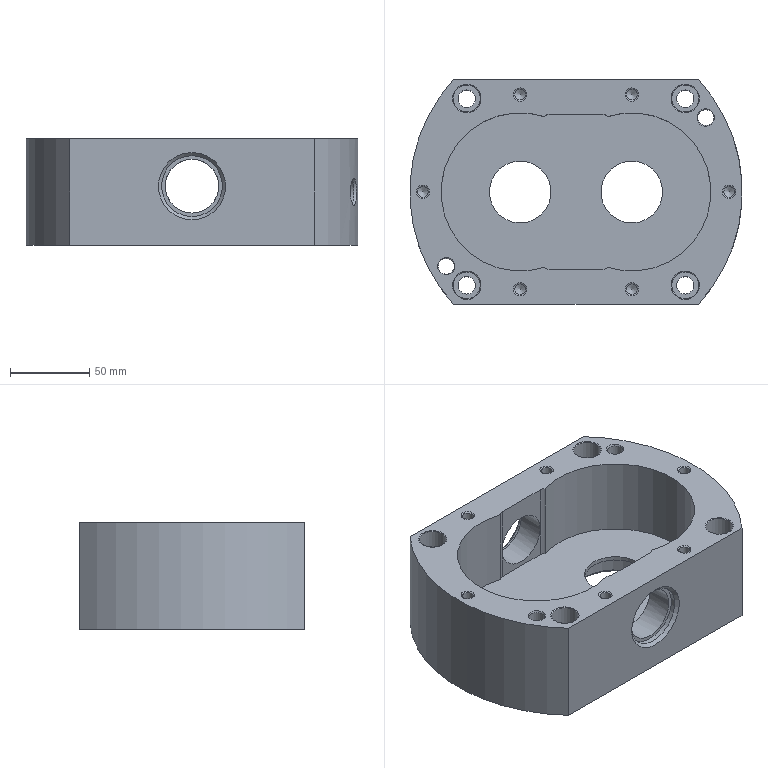NC program | NX | posted with a generic post | part box 210 x 142 x 67.4 mm
Whole program:
N10 G17 G21 G94 G90
(FLOOR_WALL , TOOL : D50)
N12 T02 M6
N14 G54
N16 G17 G0 G90 X-46.563 Y43.697 B0. C0. S1200 M3
N18 G43 Z30. H2
N20 Z2.65
N22 G94 G1 Z-0.35 F1000.
N24 X-43.563
N26 X43.563 F2000.
N28 Y9.999
N30 X-43.563
N32 Y-23.7
N34 X43.563
N36 X46.563
N38 Z2.65
N40 G0 Z30.
N42 X-50.098 Y43.697
N44 Z2.301
N46 G1 Z-0.699 F1000.
N48 X-47.098
N50 X47.098 F2000.
N52 Y9.999
N54 X-47.098
N56 Y-23.7
N58 X47.098
N60 X50.098
N62 Z2.301
N64 G0 Z30.
N66 X-52.803 Y43.697
N68 Z1.951
N70 G1 Z-1.049 F1000.
N72 X-49.803
N74 X49.803 F2000.
N76 Y9.999
N78 X-49.803
N80 Y-23.7
N82 X49.803
N84 X52.803
N86 Z1.951
N88 G0 Z30.
N90 X-55.078 Y43.697
N92 Z1.602
N94 G1 Z-1.398 F1000.
N96 X-52.078
N98 X52.078 F2000.
N100 Y9.999
N102 X-52.078
N104 Y-23.7
N106 X52.078
N108 X55.078
N110 Z1.602
N112 G0 Z30.
N114 X-57.078 Y43.697
N116 Z1.252
N118 G1 Z-1.748 F1000.
N120 X-54.078
N122 X54.078 F2000.
N124 Y9.999
N126 X-54.078
N128 Y-23.7
N130 X54.078
N132 X57.078
N134 Z1.252
N136 G0 Z30.
N138 X-58.881 Y43.697
N140 Z0.903
N142 G1 Z-2.097 F1000.
N144 X-55.881
N146 X55.881 F2000.
N148 Y9.999
N150 X-55.881
N152 Y-23.7
N154 X55.881
N156 X58.881
N158 Z0.903
N160 G0 Z30.
N162 X-60.535 Y43.697
N164 Z0.553
N166 G1 Z-2.447 F1000.
N168 X-57.535
N170 X57.535 F2000.
N172 Y9.999
N174 X-57.535
N176 Y-23.7
N178 X57.535
N180 X60.535
N182 Z0.553
N184 G0 Z30.
N186 X-62.07 Y43.697
N188 Z0.204
N190 G1 Z-2.796 F1000.
N192 X-59.07
N194 X59.07 F2000.
N196 Y9.999
N198 X-59.07
N200 Y-23.7
N202 X59.07
N204 X62.07
N206 Z0.204
N208 G0 Z30.
N210 X-63.509 Y43.697
N212 Z-0.146
N214 G1 Z-3.146 F1000.
N216 X-60.509
N218 X60.509 F2000.
N220 Y9.999
N222 X-60.509
N224 Y-23.7
N226 X60.509
N228 X63.509
N230 Z-0.146
N232 G0 Z30.
N234 X-64.866 Y43.697
N236 Z-0.495
N238 G1 Z-3.495 F1000.
N240 X-61.866
N242 X61.866 F2000.
N244 Y9.999
N246 X-61.866
N248 Y-23.7
N250 X61.866
N252 X64.866
N254 Z-0.495
N256 G0 Z30.
N258 X-66.153 Y43.697
N260 Z-0.845
N262 G1 Z-3.845 F1000.
N264 X-63.153
N266 X63.153 F2000.
N268 Y9.999
N270 X-63.153
N272 Y-23.7
N274 X63.153
N276 X66.153
N278 Z-0.845
N280 G0 Z30.
N282 X-67.38 Y43.697
N284 Z-1.194
N286 G1 Z-4.194 F1000.
N288 X-64.38
N290 X64.38 F2000.
N292 Y9.999
N294 X-64.38
N296 Y-23.7
N298 X64.38
N300 X67.38
N302 Z-1.194
N304 G0 Z30.
N306 X-68.553 Y43.697
N308 Z-1.544
N310 G1 Z-4.544 F1000.
N312 X-65.553
N314 X65.553 F2000.
N316 Y9.999
N318 X-65.553
N320 Y-23.7
N322 X65.553
N324 X68.553
N326 Z-1.544
N328 G0 Z30.
N330 X-69.68 Y43.697
N332 Z-1.893
N334 G1 Z-4.893 F1000.
N336 X-66.68
N338 X66.68 F2000.
N340 Y9.999
N342 X-66.68
N344 Y-23.7
N346 X66.68
N348 X69.68
N350 Z-1.893
N352 G0 Z30.
N354 X-70.763 Y43.697
N356 Z-2.243
N358 G1 Z-5.243 F1000.
N360 X-67.763
N362 X67.763 F2000.
N364 Y9.999
N366 X-67.763
N368 Y-23.7
N370 X67.763
N372 X70.763
N374 Z-2.243
N376 G0 Z30.
N378 X-71.809 Y43.697
N380 Z-2.592
N382 G1 Z-5.592 F1000.
N384 X-68.809
N386 X68.809 F2000.
N388 Y9.999
N390 X-68.809
N392 Y-23.7
N394 X68.809
N396 X71.809
N398 Z-2.592
N400 G0 Z30.
N402 X-72.82 Y43.697
N404 Z-2.941
N406 G1 Z-5.941 F1000.
N408 X-69.82
N410 X69.82 F2000.
N412 Y9.999
N414 X-69.82
N416 Y-23.7
N418 X69.82
N420 X72.82
N422 Z-2.941
N424 G0 Z30.
N426 X-73.798 Y43.697
N428 Z-3.291
N430 G1 Z-6.291 F1000.
N432 X-70.798
N434 X70.798 F2000.
N436 Y9.999
N438 X-70.798
N440 Y-23.7
N442 X70.798
N444 X73.798
N446 Z-3.291
N448 G0 Z30.
N450 X-74.748 Y43.697
N452 Z-3.64
N454 G1 Z-6.64 F1000.
N456 X-71.748
N458 X71.748 F2000.
N460 Y9.999
N462 X-71.748
N464 Y-23.7
N466 X71.748
N468 X74.748
N470 Z-3.64
N472 G0 Z30.
N474 X-75.67 Y43.697
N476 Z-3.99
N478 G1 Z-6.99 F1000.
N480 X-72.67
N482 X72.67 F2000.
N484 Y9.999
N486 X-72.67
N488 Y-23.7
N490 X72.67
N492 X75.67
N494 Z-3.99
N496 G0 Z30.
N498 X-76.567 Y43.697
N500 Z-4.339
N502 G1 Z-7.339 F1000.
N504 X-73.567
N506 X73.567 F2000.
N508 Y9.999
N510 X-73.567
N512 Y-23.7
N514 X73.567
N516 X76.567
N518 Z-4.339
N520 G0 Z30.
N522 X-77.44 Y43.697
N524 Z-4.689
N526 G1 Z-7.689 F1000.
N528 X-74.44
N530 X74.44 F2000.
N532 Y9.999
N534 X-74.44
N536 Y-23.7
N538 X74.44
N540 X77.44
N542 Z-4.689
N544 G0 Z30.
N546 X-78.292 Y43.697
N548 Z-5.038
N550 G1 Z-8.038 F1000.
N552 X-75.292
N554 X75.292 F2000.
N556 Y9.999
N558 X-75.292
N560 Y-23.7
N562 X75.292
N564 X78.292
N566 Z-5.038
N568 G0 Z30.
N570 X-79.123 Y43.697
N572 Z-5.388
N574 G1 Z-8.388 F1000.
N576 X-76.123
N578 X76.123 F2000.
N580 Y9.999
N582 X-76.123
N584 Y-23.7
N586 X76.123
N588 X79.123
N590 Z-5.388
N592 G0 Z30.
N594 X-79.934 Y43.697
N596 Z-5.737
N598 G1 Z-8.737 F1000.
N600 X-76.934
N602 X76.934 F2000.
N604 Y9.999
N606 X-76.934
N608 Y-23.7
N610 X76.934
N612 X79.934
N614 Z-5.737
N616 G0 Z30.
N618 X-80.728 Y43.697
N620 Z-6.087
N622 G1 Z-9.087 F1000.
N624 X-77.728
N626 X77.728 F2000.
N628 Y9.999
N630 X-77.728
N632 Y-23.7
N634 X77.728
N636 X80.728
N638 Z-6.087
N640 G0 Z30.
N642 X-81.504 Y43.697
N644 Z-6.436
N646 G1 Z-9.436 F1000.
N648 X-78.504
N650 X78.504 F2000.
N652 Y9.999
N654 X-78.504
N656 Y-23.7
N658 X78.504
N660 X81.504
N662 Z-6.436
N664 G0 Z30.
N666 X-82.263 Y43.697
N668 Z-6.786
N670 G1 Z-9.786 F1000.
N672 X-79.263
N674 X79.263 F2000.
N676 Y9.999
N678 X-79.263
N680 Y-23.7
N682 X79.263
N684 X82.263
N686 Z-6.786
N688 G0 Z30.
N690 X-83.008 Y43.697
N692 Z-7.135
N694 G1 Z-10.135 F1000.
N696 X-80.008
N698 X80.008 F2000.
N700 Y9.999
N702 X-80.008
N704 Y-23.7
N706 X80.008
N708 X83.008
N710 Z-7.135
N712 G0 Z30.
N714 X-83.737 Y43.697
N716 Z-7.485
N718 G1 Z-10.485 F1000.
N720 X-80.737
N722 X80.737 F2000.
N724 Y9.999
N726 X-80.737
N728 Y-23.7
N730 X80.737
N732 X83.737
N734 Z-7.485
N736 G0 Z30.
N738 X-84.452 Y43.697
N740 Z-7.834
N742 G1 Z-10.834 F1000.
N744 X-81.452
N746 X81.452 F2000.
N748 Y9.999
N750 X-81.452
N752 Y-23.7
N754 X81.452
N756 X84.452
N758 Z-7.834
N760 G0 Z30.
N762 X-85.154 Y43.697
N764 Z-8.184
N766 G1 Z-11.184 F1000.
N768 X-82.154
N770 X82.154 F2000.
N772 Y9.999
N774 X-82.154
N776 Y-23.7
N778 X82.154
N780 X85.154
N782 Z-8.184
N784 G0 Z30.
N786 X-85.843 Y43.697
N788 Z-8.533
N790 G1 Z-11.533 F1000.
N792 X-82.843
N794 X82.843 F2000.
N796 Y9.999
N798 X-82.843
N800 Y-23.7
N802 X82.843
N804 X85.843
N806 Z-8.533
N808 G0 Z30.
N810 X-86.52 Y43.697
N812 Z-8.883
N814 G1 Z-11.883 F1000.
N816 X-83.52
N818 X83.52 F2000.
N820 Y9.999
N822 X-83.52
N824 Y-23.7
N826 X83.52
N828 X86.52
N830 Z-8.883
N832 G0 Z30.
N834 X-87.185 Y43.697
N836 Z-9.232
N838 G1 Z-12.232 F1000.
N840 X-84.185
N842 X84.185 F2000.
N844 Y9.999
N846 X-84.185
N848 Y-23.7
N850 X84.185
N852 X87.185
N854 Z-9.232
N856 G0 Z30.
N858 X-87.838 Y43.697
N860 Z-9.582
N862 G1 Z-12.582 F1000.
N864 X-84.838
N866 X84.838 F2000.
N868 Y9.999
N870 X-84.838
N872 Y-23.7
N874 X84.838
N876 X87.838
N878 Z-9.582
N880 G0 Z30.
N882 X-88.481 Y43.697
N884 Z-9.931
N886 G1 Z-12.931 F1000.
N888 X-85.481
N890 X85.481 F2000.
N892 Y9.999
N894 X-85.481
N896 Y-23.7
N898 X85.481
N900 X88.481
N902 Z-9.931
N904 G0 Z30.
N906 X-89.113 Y43.697
N908 Z-10.281
N910 G1 Z-13.281 F1000.
N912 X-86.113
N914 X86.113 F2000.
N916 Y9.999
N918 X-86.113
N920 Y-23.7
N922 X86.113
N924 X89.113
N926 Z-10.281
N928 G0 Z30.
N930 X-89.735 Y43.697
N932 Z-10.63
N934 G1 Z-13.63 F1000.
N936 X-86.735
N938 X86.735 F2000.
N940 Y9.999
N942 X-86.735
N944 Y-23.7
N946 X86.735
N948 X89.735
N950 Z-10.63
N952 G0 Z30.
N954 X-90.348 Y43.697
N956 Z-10.98
N958 G1 Z-13.98 F1000.
N960 X-87.348
N962 X87.348 F2000.
N964 Y9.999
N966 X-87.348
N968 Y-23.7
N970 X87.348
N972 X90.348
N974 Z-10.98
N976 G0 Z30.
N978 X-90.951 Y43.697
N980 Z-11.329
N982 G1 Z-14.329 F1000.
N984 X-87.951
N986 X87.951 F2000.
N988 Y9.999
N990 X-87.951
N992 Y-23.7
N994 X87.951
N996 X90.951
N998 Z-11.329
N1000 G0 Z30.
N1002 X-91.545 Y43.697
N1004 Z-11.679
N1006 G1 Z-14.679 F1000.
N1008 X-88.545
N1010 X88.545 F2000.
N1012 Y9.999
N1014 X-88.545
N1016 Y-23.7
N1018 X88.545
N1020 X91.545
N1022 Z-11.679
N1024 G0 Z30.
N1026 X-92.13 Y43.697
N1028 Z-12.028
N1030 G1 Z-15.028 F1000.
N1032 X-89.13
N1034 X89.13 F2000.
N1036 Y9.999
N1038 X-89.13
N1040 Y-23.7
N1042 X89.13
N1044 X92.13
N1046 Z-12.028
N1048 G0 Z30.
N1050 X-92.707 Y43.697
N1052 Z-12.377
N1054 G1 Z-15.377 F1000.
N1056 X-89.707
N1058 X89.707 F2000.
N1060 Y9.999
N1062 X-89.707
N1064 Y-23.7
N1066 X89.707
N1068 X92.707
N1070 Z-12.377
N1072 G0 Z30.
N1074 X-93.275 Y43.697
N1076 Z-12.727
N1078 G1 Z-15.727 F1000.
N1080 X-90.275
N1082 X90.275 F2000.
N1084 Y9.999
N1086 X-90.275
N1088 Y-23.7
N1090 X90.275
N1092 X93.275
N1094 Z-12.727
N1096 G0 Z30.
N1098 X-93.835 Y43.697
N1100 Z-13.076
N1102 G1 Z-16.076 F1000.
N1104 X-90.835
N1106 X90.835 F2000.
N1108 Y9.999
N1110 X-90.835
N1112 Y-23.7
N1114 X90.835
N1116 X93.835
N1118 Z-13.076
N1120 G0 Z30.
N1122 X-94.388 Y43.697
N1124 Z-13.426
N1126 G1 Z-16.426 F1000.
N1128 X-91.388
N1130 X91.388 F2000.
N1132 Y9.999
N1134 X-91.388
N1136 Y-23.7
N1138 X91.388
N1140 X94.388
N1142 Z-13.426
N1144 G0 Z30.
N1146 X-94.933 Y43.697
N1148 Z-13.775
N1150 G1 Z-16.775 F1000.
N1152 X-91.933
N1154 X91.933 F2000.
N1156 Y9.999
N1158 X-91.933
N1160 Y-23.7
N1162 X91.933
N1164 X94.933
N1166 Z-13.775
N1168 G0 Z30.
N1170 X-95.471 Y43.697
N1172 Z-14.125
N1174 G1 Z-17.125 F1000.
N1176 X-92.471
N1178 X92.471 F2000.
N1180 Y9.999
N1182 X-92.471
N1184 Y-23.7
N1186 X92.471
N1188 X95.471
N1190 Z-14.125
N1192 G0 Z30.
N1194 X-96.002 Y43.697
N1196 Z-14.474
N1198 G1 Z-17.474 F1000.
N1200 X-93.002
N1202 X93.002 F2000.
N1204 Y9.999
N1206 X-93.002
N1208 Y-23.7
N1210 X93.002
N1212 X96.002
N1214 Z-14.474
N1216 G0 Z30.
N1218 X-96.526 Y43.697
N1220 Z-14.824
N1222 G1 Z-17.824 F1000.
N1224 X-93.526
N1226 X93.526 F2000.
N1228 Y9.999
N1230 X-93.526
N1232 Y-23.7
N1234 X93.526
N1236 X96.526
N1238 Z-14.824
N1240 G0 Z30.
N1242 X-97.043 Y43.697
N1244 Z-15.173
N1246 G1 Z-18.173 F1000.
N1248 X-94.043
N1250 X94.043 F2000.
N1252 Y9.999
N1254 X-94.043
N1256 Y-23.7
N1258 X94.043
N1260 X97.043
N1262 Z-15.173
N1264 G0 Z30.
N1266 X-97.554 Y43.697
N1268 Z-15.523
N1270 G1 Z-18.523 F1000.
N1272 X-94.554
N1274 X94.554 F2000.
N1276 Y9.999
N1278 X-94.554
N1280 Y-23.7
N1282 X94.554
N1284 X97.554
N1286 Z-15.523
N1288 G0 Z30.
N1290 X-98.058 Y43.697
N1292 Z-15.872
N1294 G1 Z-18.872 F1000.
N1296 X-95.058
N1298 X95.058 F2000.
N1300 Y9.999
N1302 X-95.058
N1304 Y-23.7
N1306 X95.058
N1308 X98.058
N1310 Z-15.872
N1312 G0 Z30.
N1314 X-98.557 Y43.697
N1316 Z-16.222
N1318 G1 Z-19.222 F1000.
N1320 X-95.557
N1322 X95.557 F2000.
N1324 Y9.999
N1326 X-95.557
N1328 Y-23.7
N1330 X95.557
N1332 X98.557
N1334 Z-16.222
N1336 G0 Z30.
N1338 X-99.049 Y43.697
N1340 Z-16.571
N1342 G1 Z-19.571 F1000.
N1344 X-96.049
N1346 X96.049 F2000.
N1348 Y9.999
N1350 X-96.049
N1352 Y-23.7
N1354 X96.049
N1356 X99.049
N1358 Z-16.571
N1360 G0 Z30.
N1362 X-99.535 Y43.697
N1364 Z-16.921
N1366 G1 Z-19.921 F1000.
N1368 X-96.535
N1370 X96.535 F2000.
N1372 Y9.999
N1374 X-96.535
N1376 Y-23.7
N1378 X96.535
N1380 X99.535
N1382 Z-16.921
N1384 G0 Z30.
N1386 X-100.015 Y43.697
N1388 Z-17.27
N1390 G1 Z-20.27 F1000.
N1392 X-97.015
N1394 X97.015 F2000.
N1396 Y9.999
N1398 X-97.015
N1400 Y-23.7
N1402 X97.015
N1404 X100.015
N1406 Z-17.27
N1408 G0 Z30.
N1410 X-100.49 Y43.697
N1412 Z-17.62
N1414 G1 Z-20.62 F1000.
N1416 X-97.49
N1418 X97.49 F2000.
N1420 Y9.999
N1422 X-97.49
N1424 Y-23.7
N1426 X97.49
N1428 X100.49
N1430 Z-17.62
N1432 G0 Z30.
N1434 X-100.959 Y43.697
N1436 Z-17.969
N1438 G1 Z-20.969 F1000.
N1440 X-97.959
N1442 X97.959 F2000.
N1444 Y9.999
N1446 X-97.959
N1448 Y-23.7
N1450 X97.959
N1452 X100.959
N1454 Z-17.969
N1456 G0 Z30.
N1458 X-101.423 Y43.697
N1460 Z-18.319
N1462 G1 Z-21.319 F1000.
N1464 X-98.423
N1466 X98.423 F2000.
N1468 Y9.999
N1470 X-98.423
N1472 Y-23.7
N1474 X98.423
N1476 X101.423
N1478 Z-18.319
N1480 G0 Z30.
N1482 X-101.881 Y43.697
N1484 Z-18.668
N1486 G1 Z-21.668 F1000.
N1488 X-98.881
N1490 X98.881 F2000.
N1492 Y9.999
N1494 X-98.881
N1496 Y-23.7
N1498 X98.881
N1500 X101.881
N1502 Z-18.668
N1504 G0 Z30.
N1506 X-102.334 Y43.697
N1508 Z-19.018
N1510 G1 Z-22.018 F1000.
N1512 X-99.334
N1514 X99.334 F2000.
N1516 Y9.999
N1518 X-99.334
N1520 Y-23.7
N1522 X99.334
N1524 X102.334
N1526 Z-19.018
N1528 G0 Z30.
N1530 X-102.783 Y43.697
N1532 Z-19.367
N1534 G1 Z-22.367 F1000.
N1536 X-99.783
N1538 X99.783 F2000.
N1540 Y9.999
N1542 X-99.783
N1544 Y-23.7
N1546 X99.783
N1548 X102.783
N1550 Z-19.367
N1552 G0 Z30.
N1554 X-103.226 Y43.697
N1556 Z-19.717
N1558 G1 Z-22.717 F1000.
N1560 X-100.226
N1562 X100.226 F2000.
N1564 Y9.999
N1566 X-100.226
N1568 Y-23.7
N1570 X100.226
N1572 X103.226
N1574 Z-19.717
N1576 G0 Z30.
N1578 X-103.665 Y43.697
N1580 Z-20.066
N1582 G1 Z-23.066 F1000.
N1584 X-100.665
N1586 X100.665 F2000.
N1588 Y9.999
N1590 X-100.665
N1592 Y-23.7
N1594 X100.665
N1596 X103.665
N1598 Z-20.066
N1600 G0 Z30.
N1602 X-104.098 Y43.697
N1604 Z-20.416
N1606 G1 Z-23.416 F1000.
N1608 X-101.098
N1610 X101.098 F2000.
N1612 Y9.999
N1614 X-101.098
N1616 Y-23.7
N1618 X101.098
N1620 X104.098
N1622 Z-20.416
N1624 G0 Z30.
N1626 X-104.527 Y43.697
N1628 Z-20.765
N1630 G1 Z-23.765 F1000.
N1632 X-101.527
N1634 X101.527 F2000.
N1636 Y9.999
N1638 X-101.527
N1640 Y-23.7
N1642 X101.527
N1644 X104.527
N1646 Z-20.765
N1648 G0 Z30.
N1650 X-104.952 Y43.697
N1652 Z-21.115
N1654 G1 Z-24.115 F1000.
N1656 X-101.952
N1658 X101.952 F2000.
N1660 Y9.999
N1662 X-101.952
N1664 Y-23.7
N1666 X101.952
N1668 X104.952
N1670 Z-21.115
N1672 G0 Z30.
N1674 X-105.372 Y43.697
N1676 Z-21.464
N1678 G1 Z-24.464 F1000.
N1680 X-102.372
N1682 X102.372 F2000.
N1684 Y9.999
N1686 X-102.372
N1688 Y-23.7
N1690 X102.372
N1692 X105.372
N1694 Z-21.464
N1696 G0 Z30.
N1698 X-105.787 Y43.697
N1700 Z-21.813
N1702 G1 Z-24.813 F1000.
N1704 X-102.787
N1706 X102.787 F2000.
N1708 Y9.999
N1710 X-102.787
N1712 Y-23.7
N1714 X102.787
N1716 X105.787
N1718 Z-21.813
N1720 G0 Z30.
N1722 X-106.199 Y43.697
N1724 Z-22.163
N1726 G1 Z-25.163 F1000.
N1728 X-103.199
N1730 X103.199 F2000.
N1732 Y9.999
N1734 X-103.199
N1736 Y-23.7
N1738 X103.199
N1740 X106.199
N1742 Z-22.163
N1744 G0 Z30.
N1746 X-106.606 Y43.697
N1748 Z-22.512
N1750 G1 Z-25.512 F1000.
N1752 X-103.606
N1754 X103.606 F2000.
N1756 Y9.999
N1758 X-103.606
N1760 Y-23.7
N1762 X103.606
N1764 X106.606
N1766 Z-22.512
N1768 G0 Z30.
N1770 X-107.008 Y43.697
N1772 Z-22.862
N1774 G1 Z-25.862 F1000.
N1776 X-104.008
N1778 X104.008 F2000.
N1780 Y9.999
N1782 X-104.008
N1784 Y-23.7
N1786 X104.008
N1788 X107.008
N1790 Z-22.862
N1792 G0 Z30.
N1794 X-107.407 Y43.697
N1796 Z-23.211
N1798 G1 Z-26.211 F1000.
N1800 X-104.407
N1802 X104.407 F2000.
N1804 Y9.999
N1806 X-104.407
N1808 Y-23.7
N1810 X104.407
N1812 X107.407
N1814 Z-23.211
N1816 G0 Z30.
N1818 X-107.802 Y43.697
N1820 Z-23.561
N1822 G1 Z-26.561 F1000.
N1824 X-104.802
N1826 X104.802 F2000.
N1828 Y9.999
N1830 X-104.802
N1832 Y-23.7
N1834 X104.802
N1836 X107.802
N1838 Z-23.561
N1840 G0 Z30.
N1842 X-108.193 Y43.697
N1844 Z-23.91
N1846 G1 Z-26.91 F1000.
N1848 X-105.193
N1850 X105.193 F2000.
N1852 Y9.999
N1854 X-105.193
N1856 Y-23.7
N1858 X105.193
N1860 X108.193
N1862 Z-23.91
N1864 G0 Z30.
N1866 X-108.58 Y43.697
N1868 Z-24.26
N1870 G1 Z-27.26 F1000.
N1872 X-105.58
N1874 X105.58 F2000.
N1876 Y9.999
N1878 X-105.58
N1880 Y-23.7
N1882 X105.58
N1884 X108.58
N1886 Z-24.26
N1888 G0 Z30.
N1890 X-108.963 Y43.697
N1892 Z-24.609
N1894 G1 Z-27.609 F1000.
N1896 X-105.963
N1898 X105.963 F2000.
N1900 Y9.999
N1902 X-105.963
N1904 Y-23.7
N1906 X105.963
N1908 X108.963
N1910 Z-24.609
N1912 G0 Z30.
N1914 X-109.342 Y43.697
N1916 Z-24.959
N1918 G1 Z-27.959 F1000.
N1920 X-106.342
N1922 X106.342 F2000.
N1924 Y9.999
N1926 X-106.342
N1928 Y-23.7
N1930 X106.342
N1932 X109.342
N1934 Z-24.959
N1936 G0 Z30.
N1938 X-109.717 Y43.697
N1940 Z-25.308
N1942 G1 Z-28.308 F1000.
N1944 X-106.717
N1946 X106.717 F2000.
N1948 Y9.999
N1950 X-106.717
N1952 Y-23.7
N1954 X106.717
N1956 X109.717
N1958 Z-25.308
N1960 G0 Z30.
N1962 X-110.089 Y43.697
N1964 Z-25.658
N1966 G1 Z-28.658 F1000.
N1968 X-107.089
N1970 X107.089 F2000.
N1972 Y9.999
N1974 X-107.089
N1976 Y-23.7
N1978 X107.089
N1980 X110.089
N1982 Z-25.658
N1984 G0 Z30.
N1986 X-110.458 Y43.697
N1988 Z-26.007
N1990 G1 Z-29.007 F1000.
N1992 X-107.458
N1994 X107.458 F2000.
N1996 Y9.999
N1998 X-107.458
N2000 Y-23.7
N2002 X107.458
N2004 X110.458
N2006 Z-26.007
N2008 G0 Z30.
N2010 X-110.822 Y43.697
N2012 Z-26.357
N2014 G1 Z-29.357 F1000.
N2016 X-107.822
N2018 X107.822 F2000.
N2020 Y9.999
N2022 X-107.822
N2024 Y-23.7
N2026 X107.822
N2028 X110.822
N2030 Z-26.357
N2032 G0 Z30.
N2034 X-111.184 Y43.697
N2036 Z-26.706
N2038 G1 Z-29.706 F1000.
N2040 X-108.184
N2042 X108.184 F2000.
N2044 Y9.999
N2046 X-108.184
N2048 Y-23.7
N2050 X108.184
N2052 X111.184
N2054 Z-26.706
N2056 G0 Z30.
N2058 X-111.542 Y43.697
N2060 Z-27.056
N2062 G1 Z-30.056 F1000.
N2064 X-108.542
N2066 X108.542 F2000.
N2068 Y9.999
N2070 X-108.542
N2072 Y-23.7
N2074 X108.542
N2076 X111.542
N2078 Z-27.056
N2080 G0 Z30.
N2082 X-111.896 Y43.697
N2084 Z-27.405
N2086 G1 Z-30.405 F1000.
N2088 X-108.896
N2090 X108.896 F2000.
N2092 Y9.999
N2094 X-108.896
N2096 Y-23.7
N2098 X108.896
N2100 X111.896
N2102 Z-27.405
N2104 G0 Z30.
N2106 X-112.247 Y43.697
N2108 Z-27.755
N2110 G1 Z-30.755 F1000.
N2112 X-109.247
N2114 X109.247 F2000.
N2116 Y9.999
N2118 X-109.247
N2120 Y-23.7
N2122 X109.247
N2124 X112.247
N2126 Z-27.755
N2128 G0 Z30.
N2130 X-112.595 Y43.697
N2132 Z-28.104
N2134 G1 Z-31.104 F1000.
N2136 X-109.595
N2138 X109.595 F2000.
N2140 Y9.999
N2142 X-109.595
N2144 Y-23.7
N2146 X109.595
N2148 X112.595
N2150 Z-28.104
N2152 G0 Z30.
N2154 X-112.94 Y43.697
N2156 Z-28.454
N2158 G1 Z-31.454 F1000.
N2160 X-109.94
N2162 X109.94 F2000.
N2164 Y9.999
N2166 X-109.94
N2168 Y-23.7
N2170 X109.94
N2172 X112.94
N2174 Z-28.454
N2176 G0 Z30.
N2178 X-113.281 Y43.697
N2180 Z-28.803
N2182 G1 Z-31.803 F1000.
N2184 X-110.281
N2186 X110.281 F2000.
N2188 Y9.999
N2190 X-110.281
N2192 Y-23.7
N2194 X110.281
N2196 X113.281
N2198 Z-28.803
N2200 G0 Z30.
N2202 X-113.619 Y43.697
N2204 Z-29.153
N2206 G1 Z-32.153 F1000.
N2208 X-110.619
N2210 X110.619 F2000.
N2212 Y9.999
N2214 X-110.619
N2216 Y-23.7
N2218 X110.619
N2220 X113.619
N2222 Z-29.153
N2224 G0 Z30.
N2226 X-113.954 Y43.697
N2228 Z-29.502
N2230 G1 Z-32.502 F1000.
N2232 X-110.954
N2234 X110.954 F2000.
N2236 Y9.999
N2238 X-110.954
N2240 Y-23.7
N2242 X110.954
N2244 X113.954
N2246 Z-29.502
N2248 G0 Z30.
N2250 X-114.286 Y43.697
N2252 Z-29.852
N2254 G1 Z-32.852 F1000.
N2256 X-111.286
N2258 X111.286 F2000.
N2260 Y9.999
N2262 X-111.286
N2264 Y-23.7
N2266 X111.286
N2268 X114.286
N2270 Z-29.852
N2272 G0 Z30.
N2274 X-114.615 Y43.697
N2276 Z-30.201
N2278 G1 Z-33.201 F1000.
N2280 X-111.615
N2282 X111.615 F2000.
N2284 Y9.999
N2286 X-111.615
N2288 Y-23.7
N2290 X111.615
N2292 X114.615
N2294 Z-30.201
N2296 G0 Z30.
N2298 X-114.941 Y43.697
N2300 Z-30.551
N2302 G1 Z-33.551 F1000.
N2304 X-111.941
N2306 X111.941 F2000.
N2308 Y9.999
N2310 X-111.941
N2312 Y-23.7
N2314 X111.941
N2316 X114.941
N2318 Z-30.551
N2320 G0 Z30.
N2322 X-115.264 Y43.697
N2324 Z-30.9
N2326 G1 Z-33.9 F1000.
N2328 X-112.264
N2330 X112.264 F2000.
N2332 Y9.999
N2334 X-112.264
N2336 Y-23.7
N2338 X112.264
N2340 X115.264
N2342 Z-30.9
N2344 G0 Z30.
(FLOOR_WALL_COPY , TOOL : D50)
N2346 X-115.356 Y43.697 S2500
N2348 Z-31.
N2350 G1 Z-34. F1000.
N2352 X-112.356
N2354 X112.356
N2356 Y9.999
N2358 X-112.356
N2360 Y-23.7
N2362 X112.356
N2364 X115.356
N2366 Z-31.
N2368 G0 Z30.
N2370 M5
(HOLE_MILLING , TOOL : D10)
N2372 T10 M6
N2374 G54
N2376 G17 G0 G90 X0. Y-3.7 B0. C0. S3000 M3
N2378 G43 Z30. H10
N2380 Z-35.5
N2382 G94 G3 X-1.25 Y-2.45 R1.25 F2200.
N2384 X-2.5 Y-3.7 R1.25
N2386 X-2.5 Y-3.7 Z-35.72 I2.5 J0.
N2388 X-2.5 Y-3.7 Z-35.94 I2.5 J0.
N2390 X-2.5 Y-3.7 Z-36.16 I2.5 J0.
N2392 X-2.5 Y-3.7 Z-36.38 I2.5 J0.
N2394 X-2.5 Y-3.7 Z-36.6 I2.5 J0.
N2396 X-2.5 Y-3.7 Z-36.82 I2.5 J0.
N2398 X-2.5 Y-3.7 Z-37.04 I2.5 J0.
N2400 X-2.5 Y-3.7 Z-37.26 I2.5 J0.
N2402 X-2.5 Y-3.7 Z-37.48 I2.5 J0.
N2404 X-2.5 Y-3.7 Z-37.7 I2.5 J0.
N2406 X-2.5 Y-3.7 Z-37.92 I2.5 J0.
N2408 X-2.5 Y-3.7 Z-38.14 I2.5 J0.
N2410 X-2.5 Y-3.7 Z-38.36 I2.5 J0.
N2412 X-2.5 Y-3.7 Z-38.58 I2.5 J0.
N2414 X-2.5 Y-3.7 Z-38.8 I2.5 J0.
N2416 X-2.103 Y-2.348 Z-39. R-2.5
N2418 X-1.343 Y-5.854 R2.538
N2420 X2.192 Y-5.117 R2.572
N2422 X1.462 Y-1.472 R2.63
N2424 X-2.28 Y-2.217 R2.7
N2426 X-1.528 Y-6.016 R2.74
N2428 X2.368 Y-5.249 R2.81
N2430 X1.595 Y-1.296 R2.849
N2432 X-2.456 Y-2.084 R2.919
N2434 X-1.662 Y-6.191 R2.959
N2436 X2.543 Y-5.383 R3.029
N2438 X1.729 Y-1.122 R3.069
N2440 X-2.63 Y-1.949 R3.139
N2442 X-1.797 Y-6.365 R3.179
N2444 X2.717 Y-5.519 R3.249
N2446 X1.866 Y-0.949 R3.289
N2448 X-2.803 Y-1.812 R3.359
N2450 X-1.935 Y-6.537 R3.399
N2452 X2.889 Y-5.657 R3.469
N2454 X2.004 Y-0.777 R3.509
N2456 X-2.974 Y-1.673 R3.579
N2458 X-2.074 Y-6.708 R3.619
N2460 X3.059 Y-5.797 R3.689
N2462 X2.144 Y-0.607 R3.729
N2464 X-3.144 Y-1.533 R3.799
N2466 X-2.215 Y-6.878 R3.839
N2468 X3.229 Y-5.938 R3.909
N2470 X2.286 Y-0.438 R3.949
N2472 X-3.313 Y-1.39 R4.019
N2474 X-2.358 Y-7.046 R4.058
N2476 X3.397 Y-6.082 R4.128
N2478 X2.43 Y-0.27 R4.168
N2480 X-3.48 Y-1.245 R4.238
N2482 X-2.503 Y-7.213 R4.278
N2484 X3.563 Y-6.228 R4.348
N2486 X2.576 Y-0.104 R4.388
N2488 X-3.646 Y-1.099 R4.458
N2490 X-2.65 Y-7.378 R4.498
N2492 X3.728 Y-6.375 R4.568
N2494 X2.724 Y0.06 R4.608
N2496 X-3.81 Y-0.951 R4.678
N2498 X-2.799 Y-7.542 R4.718
N2500 X3.891 Y-6.524 R4.788
N2502 X2.874 Y0.223 R4.828
N2504 X-3.972 Y-0.801 R4.898
N2506 X-2.949 Y-7.704 R4.938
N2508 X4.053 Y-6.675 R5.008
N2510 X3.025 Y0.384 R5.048
N2512 X-4.134 Y-0.649 R5.118
N2514 X-3.101 Y-7.865 R5.158
N2516 X4.214 Y-6.828 R5.228
N2518 X3.178 Y0.544 R5.267
N2520 X-4.293 Y-0.495 R5.337
N2522 X-3.256 Y-8.024 R5.377
N2524 X4.373 Y-6.982 R5.447
N2526 X3.333 Y0.703 R5.487
N2528 X-4.451 Y-0.34 R5.557
N2530 X-3.411 Y-8.182 R5.597
N2532 X4.53 Y-7.139 R5.667
N2534 X3.49 Y0.86 R5.707
N2536 X-4.608 Y-0.182 R5.777
N2538 X-3.569 Y-8.338 R5.817
N2540 X4.686 Y-7.297 R5.887
N2542 X3.649 Y1.015 R5.927
N2544 X-4.763 Y-0.023 R5.997
N2546 X-3.729 Y-8.492 R6.037
N2548 X4.84 Y-7.457 R6.107
N2550 X3.809 Y1.169 R6.147
N2552 X-4.916 Y0.138 R6.217
N2554 X-3.89 Y-8.645 R6.257
N2556 X4.992 Y-7.619 R6.327
N2558 X3.971 Y1.321 R6.367
N2560 X-5.068 Y0.3 R6.437
N2562 X-4.053 Y-8.796 R6.476
N2564 X5.143 Y-7.782 R6.546
N2566 X4.135 Y1.471 R6.586
N2568 X-5.218 Y0.465 R6.656
N2570 X-4.218 Y-8.946 R6.696
N2572 X5.293 Y-7.948 R6.766
N2574 X4.301 Y1.62 R6.806
N2576 X-5.367 Y0.631 R6.876
N2578 X-4.384 Y-9.094 R6.916
N2580 X5.44 Y-8.114 R6.986
N2582 X4.468 Y1.768 R7.026
N2584 X-5.514 Y0.799 R7.096
N2586 X-4.552 Y-9.241 R7.136
N2588 X5.587 Y-8.283 R7.206
N2590 X4.637 Y1.913 R7.246
N2592 X-5.659 Y0.968 R7.316
N2594 X-4.722 Y-9.385 R7.356
N2596 X5.731 Y-8.454 R7.426
N2598 X4.808 Y2.057 R7.466
N2600 X-5.802 Y1.139 R7.536
N2602 X-4.894 Y-9.528 R7.576
N2604 X5.874 Y-8.626 R7.646
N2606 X4.98 Y2.199 R7.685
N2608 X-5.944 Y1.312 R7.755
N2610 X-5.067 Y-9.67 R7.795
N2612 X6.015 Y-8.799 R7.865
N2614 X5.154 Y2.34 R7.905
N2616 X-6.085 Y1.487 R7.975
N2618 X-5.242 Y-9.81 R8.015
N2620 X6.154 Y-8.975 R8.085
N2622 X5.33 Y2.479 R8.125
N2624 X-6.223 Y1.663 R8.195
N2626 X-5.419 Y-9.948 R8.235
N2628 X6.292 Y-9.152 R8.305
N2630 X5.508 Y2.616 R8.345
N2632 X-6.36 Y1.841 R8.415
N2634 X-5.597 Y-10.084 R8.455
N2636 X6.427 Y-9.33 R8.525
N2638 X5.687 Y2.751 R8.565
N2640 X-6.495 Y2.02 R8.635
N2642 X-5.777 Y-10.218 R8.675
N2644 X6.562 Y-9.511 R8.745
N2646 X5.867 Y2.885 R8.785
N2648 X-6.628 Y2.201 R8.854
N2650 X-5.958 Y-10.351 R8.894
N2652 X6.694 Y-9.693 R8.964
N2654 X6.049 Y3.017 R9.004
N2656 X-6.76 Y2.384 R9.074
N2658 X-6.141 Y-10.482 R9.114
N2660 X6.825 Y-9.876 R9.184
N2662 X6.233 Y3.147 R9.224
N2664 X-6.889 Y2.568 R9.294
N2666 X-6.326 Y-10.611 R9.334
N2668 X6.953 Y-10.061 R9.404
N2670 X6.419 Y3.275 R9.444
N2672 X-7.017 Y2.754 R9.514
N2674 X-6.512 Y-10.739 R9.554
N2676 X7.08 Y-10.248 R9.624
N2678 X6.606 Y3.402 R9.664
N2680 X-7.143 Y2.942 R9.734
N2682 X-6.7 Y-10.864 R9.774
N2684 X7.206 Y-10.436 R9.844
N2686 X6.794 Y3.526 R9.884
N2688 X-7.267 Y3.131 R9.954
N2690 X-6.889 Y-10.988 R9.993
N2692 X7.329 Y-10.626 R10.063
N2694 X6.984 Y3.649 R10.103
N2696 X-7.39 Y3.321 R10.173
N2698 X-7.08 Y-11.11 R10.213
N2700 X7.45 Y-10.817 R10.283
N2702 X7.176 Y3.77 R10.323
N2704 X-7.511 Y3.513 R10.393
N2706 X-7.272 Y-11.23 R10.433
N2708 X7.57 Y-11.01 R10.503
N2710 X7.369 Y3.889 R10.543
N2712 X-7.629 Y3.706 R10.613
N2714 X-7.466 Y-11.348 R10.653
N2716 X7.688 Y-11.204 R10.723
N2718 X7.563 Y4.007 R10.763
N2720 X-7.746 Y3.901 R10.833
N2722 X-7.661 Y-11.465 R10.873
N2724 X7.804 Y-11.399 R10.943
N2726 X7.759 Y4.122 R10.983
N2728 X-7.861 Y4.098 R11.053
N2730 X-7.858 Y-11.579 R11.093
N2732 X7.918 Y-11.597 R11.163
N2734 X7.957 Y4.235 R11.202
N2736 X-7.974 Y4.296 R11.272
N2738 X-8.056 Y-11.692 R11.312
N2740 X8.03 Y-11.795 R11.382
N2742 X8.156 Y4.347 R11.422
N2744 X-8.085 Y4.495 R11.492
N2746 X-8.256 Y-11.802 R11.532
N2748 X8.14 Y-11.995 R11.602
N2750 X8.356 Y4.457 R11.642
N2752 X-8.195 Y4.696 R11.712
N2754 X-8.457 Y-11.911 R11.752
N2756 X8.249 Y-12.197 R11.822
N2758 X8.558 Y4.565 R11.862
N2760 X-8.302 Y4.898 R11.932
N2762 X-8.659 Y-12.018 R11.972
N2764 X8.355 Y-12.4 R12.042
N2766 X8.761 Y4.67 R12.082
N2768 X-8.407 Y5.102 R12.152
N2770 X-8.863 Y-12.122 R12.192
N2772 X8.459 Y-12.604 R12.262
N2774 X8.965 Y4.774 R12.302
N2776 X-8.511 Y5.306 R12.371
N2778 X-9.068 Y-12.225 R12.411
N2780 X8.562 Y-12.809 R12.481
N2782 X9.171 Y4.876 R12.521
N2784 X-8.612 Y5.513 R12.591
N2786 X-9.275 Y-12.326 R12.631
N2788 X8.662 Y-13.016 R12.701
N2790 X9.379 Y4.976 R12.741
N2792 X-8.712 Y5.72 R12.811
N2794 X-9.483 Y-12.425 R12.851
N2796 X8.761 Y-13.225 R12.921
N2798 X9.587 Y5.074 R12.961
N2800 X-8.809 Y5.929 R13.031
N2802 X-9.692 Y-12.522 R13.071
N2804 X8.857 Y-13.434 R13.141
N2806 X9.797 Y5.17 R13.181
N2808 X-8.905 Y6.14 R13.251
N2810 X-9.903 Y-12.617 R13.291
N2812 X8.952 Y-13.645 R13.361
N2814 X10.008 Y5.264 R13.401
N2816 X-8.998 Y6.351 R13.471
N2818 X-10.114 Y-12.71 R13.51
N2820 X9.044 Y-13.858 R13.58
N2822 X10.221 Y5.356 R13.62
N2824 X-9.09 Y6.564 R13.69
N2826 X-10.328 Y-12.801 R13.73
N2828 X9.134 Y-14.071 R13.8
N2830 X10.435 Y5.445 R13.84
N2832 X-9.179 Y6.778 R13.91
N2834 X-10.542 Y-12.89 R13.95
N2836 X9.223 Y-14.286 R14.02
N2838 X10.629 Y5.584 R14.078
N2840 X-9.266 Y6.994 R14.113
N2842 X-10.694 Y-12.966 R14.15
N2844 X-9.266 Y6.994 R-14.15
N2846 X-9.98 Y-2.986 R7.075
N2848 X0. Y-3.7 R7.075
N2850 G0 Z30.
(HOLE_MILLING_COPY , TOOL : D10)
N2852 Z-38.5
N2854 G3 X-1.25 Y-2.45 R1.25
N2856 X-2.5 Y-3.7 R1.25
N2858 X-2.5 Y-3.7 Z-38.72 I2.5 J0.
N2860 X-2.5 Y-3.7 Z-38.94 I2.5 J0.
N2862 X-2.5 Y-3.7 Z-39.16 I2.5 J0.
N2864 X-2.5 Y-3.7 Z-39.38 I2.5 J0.
N2866 X-2.5 Y-3.7 Z-39.6 I2.5 J0.
N2868 X-2.5 Y-3.7 Z-39.82 I2.5 J0.
N2870 X-2.5 Y-3.7 Z-40.04 I2.5 J0.
N2872 X-2.5 Y-3.7 Z-40.26 I2.5 J0.
N2874 X-2.5 Y-3.7 Z-40.48 I2.5 J0.
N2876 X-2.5 Y-3.7 Z-40.7 I2.5 J0.
N2878 X-2.5 Y-3.7 Z-40.92 I2.5 J0.
N2880 X-2.5 Y-3.7 Z-41.14 I2.5 J0.
N2882 X-2.5 Y-3.7 Z-41.36 I2.5 J0.
N2884 X-2.5 Y-3.7 Z-41.58 I2.5 J0.
N2886 X-2.5 Y-3.7 Z-41.8 I2.5 J0.
N2888 X-2.5 Y-3.7 Z-42.02 I2.5 J0.
N2890 X-2.5 Y-3.7 Z-42.24 I2.5 J0.
N2892 X-2.5 Y-3.7 Z-42.46 I2.5 J0.
N2894 X-2.5 Y-3.7 Z-42.68 I2.5 J0.
N2896 X-2.5 Y-3.7 Z-42.9 I2.5 J0.
N2898 X-2.5 Y-3.7 Z-43.12 I2.5 J0.
N2900 X-2.5 Y-3.7 Z-43.34 I2.5 J0.
N2902 X-2.5 Y-3.7 Z-43.56 I2.5 J0.
N2904 X-2.5 Y-3.7 Z-43.78 I2.5 J0.
N2906 X-2.5 Y-3.7 Z-44. I2.5 J0.
N2908 X-2.5 Y-3.7 Z-44.22 I2.5 J0.
N2910 X-2.5 Y-3.7 Z-44.44 I2.5 J0.
N2912 X-2.5 Y-3.7 Z-44.66 I2.5 J0.
N2914 X-2.5 Y-3.7 Z-44.88 I2.5 J0.
N2916 X-2.5 Y-3.7 Z-45.1 I2.5 J0.
N2918 X-2.5 Y-3.7 Z-45.32 I2.5 J0.
N2920 X-2.5 Y-3.7 Z-45.54 I2.5 J0.
N2922 X-2.5 Y-3.7 Z-45.76 I2.5 J0.
N2924 X-2.5 Y-3.7 Z-45.98 I2.5 J0.
N2926 X-2.5 Y-3.7 Z-46.2 I2.5 J0.
N2928 X-2.5 Y-3.7 Z-46.42 I2.5 J0.
N2930 X-2.5 Y-3.7 Z-46.64 I2.5 J0.
N2932 X-2.5 Y-3.7 Z-46.86 I2.5 J0.
N2934 X-2.5 Y-3.7 Z-47.08 I2.5 J0.
N2936 X-2.5 Y-3.7 Z-47.3 I2.5 J0.
N2938 X-2.5 Y-3.7 Z-47.52 I2.5 J0.
N2940 X-2.5 Y-3.7 Z-47.74 I2.5 J0.
N2942 X-2.5 Y-3.7 Z-47.96 I2.5 J0.
N2944 X-2.5 Y-3.7 Z-48.18 I2.5 J0.
N2946 X-2.5 Y-3.7 Z-48.4 I2.5 J0.
N2948 X-2.5 Y-3.7 Z-48.62 I2.5 J0.
N2950 X-2.5 Y-3.7 Z-48.84 I2.5 J0.
N2952 X-2.5 Y-3.7 Z-49.06 I2.5 J0.
N2954 X-2.5 Y-3.7 Z-49.28 I2.5 J0.
N2956 X-2.5 Y-3.7 Z-49.5 I2.5 J0.
N2958 X-2.5 Y-3.7 Z-49.72 I2.5 J0.
N2960 X-2.5 Y-3.7 Z-49.94 I2.5 J0.
N2962 X-2.5 Y-3.7 Z-50.16 I2.5 J0.
N2964 X-2.5 Y-3.7 Z-50.38 I2.5 J0.
N2966 X-2.5 Y-3.7 Z-50.6 I2.5 J0.
N2968 X-2.5 Y-3.7 Z-50.82 I2.5 J0.
N2970 X-2.5 Y-3.7 Z-51.04 I2.5 J0.
N2972 X-2.5 Y-3.7 Z-51.26 I2.5 J0.
N2974 X-2.5 Y-3.7 Z-51.48 I2.5 J0.
N2976 X-2.5 Y-3.7 Z-51.7 I2.5 J0.
N2978 X-2.5 Y-3.7 Z-51.92 I2.5 J0.
N2980 X-2.5 Y-3.7 Z-52.14 I2.5 J0.
N2982 X-2.5 Y-3.7 Z-52.36 I2.5 J0.
N2984 X-2.5 Y-3.7 Z-52.58 I2.5 J0.
N2986 X-2.5 Y-3.7 Z-52.8 I2.5 J0.
N2988 X-2.5 Y-3.7 Z-53.02 I2.5 J0.
N2990 X-2.5 Y-3.7 Z-53.24 I2.5 J0.
N2992 X-2.5 Y-3.7 Z-53.46 I2.5 J0.
N2994 X-2.5 Y-3.7 Z-53.68 I2.5 J0.
N2996 X-2.5 Y-3.7 Z-53.9 I2.5 J0.
N2998 X-2.5 Y-3.7 Z-54.12 I2.5 J0.
N3000 X-2.5 Y-3.7 Z-54.34 I2.5 J0.
N3002 X-2.5 Y-3.7 Z-54.56 I2.5 J0.
N3004 X-2.5 Y-3.7 Z-54.78 I2.5 J0.
N3006 X-2.5 Y-3.7 Z-55. I2.5 J0.
N3008 X-2.5 Y-3.7 Z-55.22 I2.5 J0.
N3010 X-2.5 Y-3.7 Z-55.44 I2.5 J0.
N3012 X-2.5 Y-3.7 Z-55.66 I2.5 J0.
N3014 X-2.5 Y-3.7 Z-55.88 I2.5 J0.
N3016 X-2.5 Y-3.7 Z-56.1 I2.5 J0.
N3018 X-2.5 Y-3.7 Z-56.32 I2.5 J0.
N3020 X-2.5 Y-3.7 Z-56.54 I2.5 J0.
N3022 X-2.5 Y-3.7 Z-56.76 I2.5 J0.
N3024 X-2.5 Y-3.7 Z-56.98 I2.5 J0.
N3026 X-2.5 Y-3.7 Z-57.2 I2.5 J0.
N3028 X-2.5 Y-3.7 Z-57.42 I2.5 J0.
N3030 X1.637 Y-5.589 Z-57.5 R2.5
N3032 X1.893 Y-2.014 R2.534
N3034 X-1.703 Y-1.735 R2.566
N3036 X-2.012 Y-5.425 R2.618
N3038 X1.768 Y-5.741 R2.682
N3040 X2.087 Y-1.91 R2.718
N3042 X-1.834 Y-1.584 R2.782
N3044 X-2.163 Y-5.556 R2.818
N3046 X1.899 Y-5.892 R2.882
N3048 X2.238 Y-1.779 R2.918
N3050 X-1.965 Y-1.433 R2.982
N3052 X-2.314 Y-5.687 R3.018
N3054 X2.03 Y-6.043 R3.082
N3056 X2.389 Y-1.648 R3.118
N3058 X-2.096 Y-1.282 R3.182
N3060 X-2.465 Y-5.818 R3.218
N3062 X2.161 Y-6.194 R3.282
N3064 X2.541 Y-1.517 R3.318
N3066 X-2.227 Y-1.13 R3.382
N3068 X-2.616 Y-5.949 R3.418
N3070 X2.292 Y-6.345 R3.482
N3072 X2.692 Y-1.386 R3.518
N3074 X-2.357 Y-0.979 R3.582
N3076 X-2.767 Y-6.08 R3.618
N3078 X2.423 Y-6.496 R3.682
N3080 X2.843 Y-1.255 R3.718
N3082 X-2.488 Y-0.828 R3.782
N3084 X-2.919 Y-6.211 R3.818
N3086 X2.554 Y-6.647 R3.882
N3088 X2.994 Y-1.124 R3.918
N3090 X-2.619 Y-0.677 R3.982
N3092 X-3.07 Y-6.342 R4.018
N3094 X2.685 Y-6.799 R4.082
N3096 X3.145 Y-0.993 R4.118
N3098 X-2.75 Y-0.526 R4.182
N3100 X-3.221 Y-6.473 R4.218
N3102 X2.816 Y-6.95 R4.282
N3104 X3.296 Y-0.862 R4.318
N3106 X-2.881 Y-0.375 R4.382
N3108 X-3.372 Y-6.604 R4.418
N3110 X2.947 Y-7.101 R4.482
N3112 X3.448 Y-0.731 R4.518
N3114 X-3.012 Y-0.224 R4.582
N3116 X-3.523 Y-6.735 R4.618
N3118 X3.078 Y-7.252 R4.682
N3120 X3.599 Y-0.6 R4.718
N3122 X-3.143 Y-0.072 R4.782
N3124 X-3.674 Y-6.866 R4.818
N3126 X3.209 Y-7.403 R4.882
N3128 X3.75 Y-0.469 R4.918
N3130 X-3.274 Y0.079 R4.982
N3132 X-3.825 Y-6.997 R5.018
N3134 X3.34 Y-7.554 R5.082
N3136 X3.901 Y-0.338 R5.118
N3138 X-3.405 Y0.23 R5.182
N3140 X-3.977 Y-7.128 R5.218
N3142 X3.471 Y-7.705 R5.282
N3144 X4.052 Y-0.207 R5.318
N3146 X-3.536 Y0.381 R5.382
N3148 X-4.128 Y-7.259 R5.418
N3150 X3.602 Y-7.857 R5.482
N3152 X4.203 Y-0.076 R5.518
N3154 X-3.667 Y0.532 R5.582
N3156 X-4.279 Y-7.39 R5.618
N3158 X3.733 Y-8.008 R5.682
N3160 X4.354 Y0.055 R5.718
N3162 X-3.798 Y0.683 R5.782
N3164 X-4.43 Y-7.521 R5.818
N3166 X3.864 Y-8.159 R5.882
N3168 X4.506 Y0.186 R5.918
N3170 X-3.929 Y0.834 R5.982
N3172 X-4.581 Y-7.652 R6.018
N3174 X3.995 Y-8.31 R6.082
N3176 X4.657 Y0.317 R6.118
N3178 X-4.06 Y0.986 R6.182
N3180 X-4.732 Y-7.783 R6.218
N3182 X4.126 Y-8.461 R6.282
N3184 X4.808 Y0.448 R6.318
N3186 X-4.191 Y1.137 R6.382
N3188 X-4.883 Y-7.913 R6.418
N3190 X4.257 Y-8.612 R6.482
N3192 X4.959 Y0.579 R6.518
N3194 X-4.322 Y1.288 R6.582
N3196 X-5.035 Y-8.044 R6.618
N3198 X4.388 Y-8.764 R6.682
N3200 X5.11 Y0.71 R6.718
N3202 X-4.453 Y1.439 R6.782
N3204 X-5.186 Y-8.175 R6.818
N3206 X4.519 Y-8.915 R6.882
N3208 X5.261 Y0.841 R6.918
N3210 X-4.584 Y1.59 R6.982
N3212 X-5.337 Y-8.306 R7.018
N3214 X4.65 Y-9.066 R7.082
N3216 X5.413 Y0.972 R7.118
N3218 X-4.715 Y1.741 R7.182
N3220 X-5.488 Y-8.437 R7.218
N3222 X4.78 Y-9.217 R7.282
N3224 X5.564 Y1.103 R7.318
N3226 X-4.846 Y1.893 R7.382
N3228 X-5.639 Y-8.568 R7.418
N3230 X4.911 Y-9.368 R7.482
N3232 X5.715 Y1.234 R7.518
N3234 X-4.977 Y2.044 R7.582
N3236 X-5.79 Y-8.699 R7.618
N3238 X5.042 Y-9.519 R7.682
N3240 X5.866 Y1.365 R7.718
N3242 X-5.108 Y2.195 R7.782
N3244 X-5.942 Y-8.83 R7.818
N3246 X5.173 Y-9.67 R7.882
N3248 X6.017 Y1.496 R7.918
N3250 X-5.239 Y2.346 R7.982
N3252 X-6.093 Y-8.961 R8.018
N3254 X5.304 Y-9.822 R8.082
N3256 X6.168 Y1.627 R8.118
N3258 X-5.37 Y2.497 R8.182
N3260 X-6.244 Y-9.092 R8.218
N3262 X5.435 Y-9.973 R8.282
N3264 X6.319 Y1.758 R8.318
N3266 X-5.501 Y2.648 R8.382
N3268 X-6.395 Y-9.223 R8.418
N3270 X5.566 Y-10.124 R8.482
N3272 X6.471 Y1.889 R8.518
N3274 X-5.632 Y2.799 R8.582
N3276 X-6.546 Y-9.354 R8.618
N3278 X5.697 Y-10.275 R8.682
N3280 X6.622 Y2.02 R8.718
N3282 X-5.763 Y2.951 R8.782
N3284 X-6.697 Y-9.485 R8.818
N3286 X5.828 Y-10.426 R8.882
N3288 X6.773 Y2.151 R8.918
N3290 X-5.894 Y3.102 R8.982
N3292 X-6.848 Y-9.616 R9.018
N3294 X5.959 Y-10.577 R9.082
N3296 X6.924 Y2.282 R9.118
N3298 X-6.025 Y3.253 R9.182
N3300 X-7. Y-9.747 R9.218
N3302 X6.09 Y-10.728 R9.282
N3304 X7.075 Y2.413 R9.318
N3306 X-6.156 Y3.404 R9.382
N3308 X-7.151 Y-9.878 R9.418
N3310 X6.221 Y-10.88 R9.482
N3312 X7.226 Y2.544 R9.518
N3314 X-6.287 Y3.555 R9.582
N3316 X-7.302 Y-10.009 R9.618
N3318 X6.352 Y-11.031 R9.682
N3320 X7.377 Y2.675 R9.718
N3322 X-6.418 Y3.706 R9.782
N3324 X-7.453 Y-10.14 R9.818
N3326 X6.483 Y-11.182 R9.882
N3328 X7.529 Y2.806 R9.918
N3330 X-6.549 Y3.857 R9.982
N3332 X-7.604 Y-10.271 R10.018
N3334 X6.614 Y-11.333 R10.082
N3336 X7.68 Y2.936 R10.118
N3338 X-6.68 Y4.009 R10.182
N3340 X-7.755 Y-10.402 R10.218
N3342 X6.745 Y-11.484 R10.282
N3344 X7.831 Y3.067 R10.318
N3346 X-6.811 Y4.16 R10.382
N3348 X-7.906 Y-10.533 R10.418
N3350 X6.876 Y-11.635 R10.482
N3352 X7.982 Y3.198 R10.518
N3354 X-6.942 Y4.311 R10.582
N3356 X-8.058 Y-10.664 R10.618
N3358 X7.007 Y-11.787 R10.682
N3360 X8.133 Y3.329 R10.718
N3362 X-7.072 Y4.462 R10.782
N3364 X-8.209 Y-10.795 R10.818
N3366 X7.138 Y-11.938 R10.882
N3368 X8.284 Y3.46 R10.918
N3370 X-7.203 Y4.613 R10.982
N3372 X-8.36 Y-10.926 R11.018
N3374 X7.269 Y-12.089 R11.082
N3376 X8.436 Y3.591 R11.118
N3378 X-7.334 Y4.764 R11.182
N3380 X-8.511 Y-11.057 R11.218
N3382 X7.4 Y-12.24 R11.282
N3384 X8.587 Y3.722 R11.318
N3386 X-7.465 Y4.916 R11.382
N3388 X-8.662 Y-11.188 R11.418
N3390 X7.531 Y-12.391 R11.482
N3392 X8.738 Y3.853 R11.518
N3394 X-7.596 Y5.067 R11.582
N3396 X-8.813 Y-11.319 R11.618
N3398 X7.662 Y-12.542 R11.682
N3400 X8.889 Y3.984 R11.718
N3402 X-7.727 Y5.218 R11.782
N3404 X-8.945 Y-11.496 R11.834
N3406 X7.793 Y-12.693 R11.866
N3408 X8.993 Y4.093 R11.9
N3410 X7.793 Y-12.693 R-11.9
N3412 X8.393 Y-4.3 R5.95
N3414 X0. Y-3.7 R5.95
N3416 G0 Z30.
N3418 M5
(HOLE_MILLING_COPY_1 , TOOL : D10JING)
N3420 T11 M6
N3422 G54
N3424 G17 G0 G90 X0. Y-3.7 B0. C0. S5000 M3
N3426 G43 Z30. H11
N3428 Z-39.
N3430 G94 G1 X-10.823 Y-1.018 F1000.
N3432 G3 X-14.25 Y-3.7 R2.763
N3434 X0. Y-17.95 R14.25
N3436 X-14.25 Y-3.7 R-14.25
N3438 X-10.823 Y-6.382 R2.763
N3440 G1 X0. Y-3.7
N3442 G0 Z30.
(HOLE_MILLING_COPY_1_COPY , TOOL : D10JING)
N3444 Z-56.
N3446 G3 X-6. Y2.3 R6.
N3448 X-12. Y-3.7 R6.
N3450 X0. Y-15.7 R12.
N3452 X-12. Y-3.7 R-12.
N3454 X-6. Y-9.7 R6.
N3456 X0. Y-3.7 R6.
N3458 G0 Z30.
N3460 M5
(PLANAR_MILL , TOOL : D6A45)
N3462 T07 M6
N3464 G54
N3466 G17 G0 G90 X78.83 Y-35.4 B0. C0. S7500 M3
N3468 G43 Z30. H7
N3470 Z-32.
N3472 G94 G1 Z-35. F1250.
N3474 X78.122 Y-34.557
N3476 G3 X77.356 Y-34.2 R1.
N3478 G1 X-77.356
N3480 G3 X-78.122 Y-34.557 R1.
N3482 G1 X-78.83 Y-35.4
N3484 Z-32.
N3486 G0 Z30.
N3488 Y35.4
N3490 Z-32.
N3492 G1 Z-35.
N3494 X-78.122 Y34.557
N3496 G3 X-77.356 Y34.2 R1.
N3498 G1 X77.356
N3500 G3 X78.122 Y34.557 R1.
N3502 G1 X78.83 Y35.4
N3504 Z-32.
N3506 G0 Z30.
(PLANAR_MILL_COPY , TOOL : D6A45)
N3508 X-1.533 Y-20.179
N3510 Z-33.5
N3512 G1 Z-36.5
N3514 X-0.766 Y-21.093
N3516 G3 X0. Y-21.45 R1.
N3518 X17.75 Y-3.7 R17.75
N3520 X0. Y-21.45 R-17.75
N3522 X0.766 Y-21.093 R1.
N3524 G1 X-0.766 Y-21.593
N3526 G3 X0. Y-21.95 R1.
N3528 X18.25 Y-3.7 R18.25
N3530 X0. Y-21.95 R-18.25
N3532 X0.766 Y-21.593 R1.
N3534 G1 X-0.766 Y-22.093
N3536 G3 X0. Y-22.45 R1.
N3538 X18.75 Y-3.7 R18.75
N3540 X0. Y-22.45 R-18.75
N3542 X0.766 Y-22.093 R1.
N3544 G1 X1.529 Y-21.183
N3546 Z-33.5
N3548 G0 Z30.
N3550 M5
N3552 M2